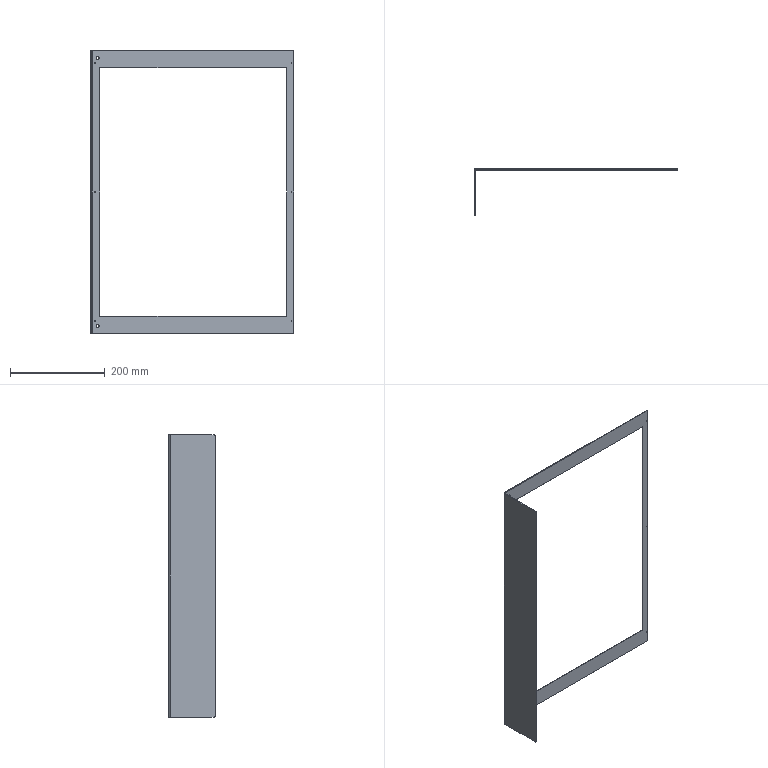Part | NX | features solid 2 | 1 solid | 32 faces | box 430 x 98 x 596 mm | volume 209789 mm3 | cylinder 20 | plane 12 | commonest cylinder face diameters 1 x12 6 x4 5 x2 4 x1 8 x1
STEP:
#1=CARTESIAN_POINT('',(-870.,-1585.,662.5));
#2=VERTEX_POINT('',#1);
#3=CARTESIAN_POINT('',(-870.,-1587.,662.5));
#4=VERTEX_POINT('',#3);
#5=CARTESIAN_POINT('',(-870.,-845.569,662.5));
#6=DIRECTION('',(0.,-1.,0.));
#7=VECTOR('',#6,1000.);
#8=LINE('',#5,#7);
#9=EDGE_CURVE('',#2,#4,#8,.T.);
#10=ORIENTED_EDGE('',*,*,#9,.F.);
#11=CARTESIAN_POINT('',(-870.,-1585.,661.5));
#12=VERTEX_POINT('',#11);
#13=CARTESIAN_POINT('',(-870.,-1585.,662.));
#14=DIRECTION('',(0.,-1.,0.));
#15=DIRECTION('',(0.,0.,-1.));
#16=AXIS2_PLACEMENT_3D('',#13,#14,#15);
#17=CIRCLE('',#16,0.5);
#18=EDGE_CURVE('',#12,#2,#17,.T.);
#19=ORIENTED_EDGE('',*,*,#18,.F.);
#20=CARTESIAN_POINT('',(-870.,-1587.,661.5));
#21=VERTEX_POINT('',#20);
#22=CARTESIAN_POINT('',(-870.,-845.569,661.5));
#23=DIRECTION('',(0.,-1.,0.));
#24=VECTOR('',#23,1000.);
#25=LINE('',#22,#24);
#26=EDGE_CURVE('',#21,#12,#25,.F.);
#27=ORIENTED_EDGE('',*,*,#26,.F.);
#28=CARTESIAN_POINT('',(-870.,-1587.,662.));
#29=DIRECTION('',(0.,-1.,0.));
#30=DIRECTION('',(1.,0.,0.));
#31=AXIS2_PLACEMENT_3D('',#28,#29,#30);
#32=CIRCLE('',#31,0.5);
#33=EDGE_CURVE('',#21,#4,#32,.T.);
#34=ORIENTED_EDGE('',*,*,#33,.T.);
#35=EDGE_LOOP('',(#10,#19,#27,#34));
#36=FACE_BOUND('',#35,.T.);
#37=CARTESIAN_POINT('',(-870.,-845.569,662.));
#38=DIRECTION('',(0.,-1.,0.));
#39=DIRECTION('',(0.,0.,-1.));
#40=AXIS2_PLACEMENT_3D('',#37,#38,#39);
#41=CYLINDRICAL_SURFACE('',#40,0.5);
#42=ADVANCED_FACE('',(#36),#41,.F.);
#43=CARTESIAN_POINT('',(-455.,-1585.,662.5));
#44=VERTEX_POINT('',#43);
#45=CARTESIAN_POINT('',(-455.,-1587.,662.5));
#46=VERTEX_POINT('',#45);
#47=CARTESIAN_POINT('',(-455.,-845.569,662.5));
#48=DIRECTION('',(0.,-1.,0.));
#49=VECTOR('',#48,1000.);
#50=LINE('',#47,#49);
#51=EDGE_CURVE('',#44,#46,#50,.T.);
#52=ORIENTED_EDGE('',*,*,#51,.F.);
#53=CARTESIAN_POINT('',(-455.,-1585.,661.5));
#54=VERTEX_POINT('',#53);
#55=CARTESIAN_POINT('',(-455.,-1585.,662.));
#56=DIRECTION('',(0.,-1.,0.));
#57=DIRECTION('',(0.,0.,-1.));
#58=AXIS2_PLACEMENT_3D('',#55,#56,#57);
#59=CIRCLE('',#58,0.5);
#60=EDGE_CURVE('',#54,#44,#59,.T.);
#61=ORIENTED_EDGE('',*,*,#60,.F.);
#62=CARTESIAN_POINT('',(-455.,-1587.,661.5));
#63=VERTEX_POINT('',#62);
#64=CARTESIAN_POINT('',(-455.,-845.569,661.5));
#65=DIRECTION('',(0.,-1.,0.));
#66=VECTOR('',#65,1000.);
#67=LINE('',#64,#66);
#68=EDGE_CURVE('',#63,#54,#67,.F.);
#69=ORIENTED_EDGE('',*,*,#68,.F.);
#70=CARTESIAN_POINT('',(-455.,-1587.,662.));
#71=DIRECTION('',(0.,-1.,0.));
#72=DIRECTION('',(1.,0.,0.));
#73=AXIS2_PLACEMENT_3D('',#70,#71,#72);
#74=CIRCLE('',#73,0.5);
#75=EDGE_CURVE('',#63,#46,#74,.T.);
#76=ORIENTED_EDGE('',*,*,#75,.T.);
#77=EDGE_LOOP('',(#52,#61,#69,#76));
#78=FACE_BOUND('',#77,.T.);
#79=CARTESIAN_POINT('',(-455.,-845.569,662.));
#80=DIRECTION('',(0.,-1.,0.));
#81=DIRECTION('',(0.,0.,-1.));
#82=AXIS2_PLACEMENT_3D('',#79,#80,#81);
#83=CYLINDRICAL_SURFACE('',#82,0.5);
#84=ADVANCED_FACE('',(#78),#83,.F.);
#85=CARTESIAN_POINT('',(-870.,-1587.,935.5));
#86=VERTEX_POINT('',#85);
#87=CARTESIAN_POINT('',(-870.,-1585.,935.5));
#88=VERTEX_POINT('',#87);
#89=CARTESIAN_POINT('',(-870.,-845.569,935.5));
#90=DIRECTION('',(0.,-1.,0.));
#91=VECTOR('',#90,1000.);
#92=LINE('',#89,#91);
#93=EDGE_CURVE('',#86,#88,#92,.F.);
#94=ORIENTED_EDGE('',*,*,#93,.T.);
#95=CARTESIAN_POINT('',(-870.,-1585.,934.5));
#96=VERTEX_POINT('',#95);
#97=CARTESIAN_POINT('',(-870.,-1585.,935.));
#98=DIRECTION('',(0.,-1.,0.));
#99=DIRECTION('',(0.,0.,-1.));
#100=AXIS2_PLACEMENT_3D('',#97,#98,#99);
#101=CIRCLE('',#100,0.5);
#102=EDGE_CURVE('',#96,#88,#101,.T.);
#103=ORIENTED_EDGE('',*,*,#102,.F.);
#104=CARTESIAN_POINT('',(-870.,-1587.,934.5));
#105=VERTEX_POINT('',#104);
#106=CARTESIAN_POINT('',(-870.,-845.569,934.5));
#107=DIRECTION('',(0.,-1.,0.));
#108=VECTOR('',#107,1000.);
#109=LINE('',#106,#108);
#110=EDGE_CURVE('',#96,#105,#109,.T.);
#111=ORIENTED_EDGE('',*,*,#110,.T.);
#112=CARTESIAN_POINT('',(-870.,-1587.,935.));
#113=DIRECTION('',(0.,-1.,0.));
#114=DIRECTION('',(1.,0.,0.));
#115=AXIS2_PLACEMENT_3D('',#112,#113,#114);
#116=CIRCLE('',#115,0.5);
#117=EDGE_CURVE('',#105,#86,#116,.T.);
#118=ORIENTED_EDGE('',*,*,#117,.T.);
#119=EDGE_LOOP('',(#94,#103,#111,#118));
#120=FACE_BOUND('',#119,.T.);
#121=CARTESIAN_POINT('',(-870.,-845.569,935.));
#122=DIRECTION('',(0.,-1.,0.));
#123=DIRECTION('',(0.,0.,-1.));
#124=AXIS2_PLACEMENT_3D('',#121,#122,#123);
#125=CYLINDRICAL_SURFACE('',#124,0.5);
#126=ADVANCED_FACE('',(#120),#125,.F.);
#127=CARTESIAN_POINT('',(-455.,-1585.,935.5));
#128=VERTEX_POINT('',#127);
#129=CARTESIAN_POINT('',(-455.,-1587.,935.5));
#130=VERTEX_POINT('',#129);
#131=CARTESIAN_POINT('',(-455.,-845.569,935.5));
#132=DIRECTION('',(0.,-1.,0.));
#133=VECTOR('',#132,1000.);
#134=LINE('',#131,#133);
#135=EDGE_CURVE('',#128,#130,#134,.T.);
#136=ORIENTED_EDGE('',*,*,#135,.F.);
#137=CARTESIAN_POINT('',(-455.,-1585.,934.5));
#138=VERTEX_POINT('',#137);
#139=CARTESIAN_POINT('',(-455.,-1585.,935.));
#140=DIRECTION('',(0.,-1.,0.));
#141=DIRECTION('',(0.,0.,-1.));
#142=AXIS2_PLACEMENT_3D('',#139,#140,#141);
#143=CIRCLE('',#142,0.5);
#144=EDGE_CURVE('',#138,#128,#143,.T.);
#145=ORIENTED_EDGE('',*,*,#144,.F.);
#146=CARTESIAN_POINT('',(-455.,-1587.,934.5));
#147=VERTEX_POINT('',#146);
#148=CARTESIAN_POINT('',(-455.,-845.569,934.5));
#149=DIRECTION('',(0.,-1.,0.));
#150=VECTOR('',#149,1000.);
#151=LINE('',#148,#150);
#152=EDGE_CURVE('',#147,#138,#151,.F.);
#153=ORIENTED_EDGE('',*,*,#152,.F.);
#154=CARTESIAN_POINT('',(-455.,-1587.,935.));
#155=DIRECTION('',(0.,-1.,0.));
#156=DIRECTION('',(1.,0.,0.));
#157=AXIS2_PLACEMENT_3D('',#154,#155,#156);
#158=CIRCLE('',#157,0.5);
#159=EDGE_CURVE('',#147,#130,#158,.T.);
#160=ORIENTED_EDGE('',*,*,#159,.T.);
#161=EDGE_LOOP('',(#136,#145,#153,#160));
#162=FACE_BOUND('',#161,.T.);
#163=CARTESIAN_POINT('',(-455.,-845.569,935.));
#164=DIRECTION('',(0.,-1.,0.));
#165=DIRECTION('',(0.,0.,-1.));
#166=AXIS2_PLACEMENT_3D('',#163,#164,#165);
#167=CYLINDRICAL_SURFACE('',#166,0.5);
#168=ADVANCED_FACE('',(#162),#167,.F.);
#169=CARTESIAN_POINT('',(-455.,-1585.,389.5));
#170=VERTEX_POINT('',#169);
#171=CARTESIAN_POINT('',(-455.,-1587.,389.5));
#172=VERTEX_POINT('',#171);
#173=CARTESIAN_POINT('',(-455.,-845.569,389.5));
#174=DIRECTION('',(0.,-1.,0.));
#175=VECTOR('',#174,1000.);
#176=LINE('',#173,#175);
#177=EDGE_CURVE('',#170,#172,#176,.T.);
#178=ORIENTED_EDGE('',*,*,#177,.F.);
#179=CARTESIAN_POINT('',(-455.,-1585.,388.5));
#180=VERTEX_POINT('',#179);
#181=CARTESIAN_POINT('',(-455.,-1585.,389.));
#182=DIRECTION('',(0.,-1.,0.));
#183=DIRECTION('',(0.,0.,-1.));
#184=AXIS2_PLACEMENT_3D('',#181,#182,#183);
#185=CIRCLE('',#184,0.5);
#186=EDGE_CURVE('',#180,#170,#185,.T.);
#187=ORIENTED_EDGE('',*,*,#186,.F.);
#188=CARTESIAN_POINT('',(-455.,-1587.,388.5));
#189=VERTEX_POINT('',#188);
#190=CARTESIAN_POINT('',(-455.,-845.569,388.5));
#191=DIRECTION('',(0.,-1.,0.));
#192=VECTOR('',#191,1000.);
#193=LINE('',#190,#192);
#194=EDGE_CURVE('',#189,#180,#193,.F.);
#195=ORIENTED_EDGE('',*,*,#194,.F.);
#196=CARTESIAN_POINT('',(-455.,-1587.,389.));
#197=DIRECTION('',(0.,-1.,0.));
#198=DIRECTION('',(1.,0.,0.));
#199=AXIS2_PLACEMENT_3D('',#196,#197,#198);
#200=CIRCLE('',#199,0.5);
#201=EDGE_CURVE('',#189,#172,#200,.T.);
#202=ORIENTED_EDGE('',*,*,#201,.T.);
#203=EDGE_LOOP('',(#178,#187,#195,#202));
#204=FACE_BOUND('',#203,.T.);
#205=CARTESIAN_POINT('',(-455.,-845.569,389.));
#206=DIRECTION('',(0.,-1.,0.));
#207=DIRECTION('',(0.,0.,-1.));
#208=AXIS2_PLACEMENT_3D('',#205,#206,#207);
#209=CYLINDRICAL_SURFACE('',#208,0.5);
#210=ADVANCED_FACE('',(#204),#209,.F.);
#211=CARTESIAN_POINT('',(-870.,-1585.,389.5));
#212=VERTEX_POINT('',#211);
#213=CARTESIAN_POINT('',(-870.,-1587.,389.5));
#214=VERTEX_POINT('',#213);
#215=CARTESIAN_POINT('',(-870.,-845.569,389.5));
#216=DIRECTION('',(0.,-1.,0.));
#217=VECTOR('',#216,1000.);
#218=LINE('',#215,#217);
#219=EDGE_CURVE('',#212,#214,#218,.T.);
#220=ORIENTED_EDGE('',*,*,#219,.F.);
#221=CARTESIAN_POINT('',(-870.,-1585.,388.5));
#222=VERTEX_POINT('',#221);
#223=CARTESIAN_POINT('',(-870.,-1585.,389.));
#224=DIRECTION('',(0.,-1.,0.));
#225=DIRECTION('',(0.,0.,-1.));
#226=AXIS2_PLACEMENT_3D('',#223,#224,#225);
#227=CIRCLE('',#226,0.5);
#228=EDGE_CURVE('',#222,#212,#227,.T.);
#229=ORIENTED_EDGE('',*,*,#228,.F.);
#230=CARTESIAN_POINT('',(-870.,-1587.,388.5));
#231=VERTEX_POINT('',#230);
#232=CARTESIAN_POINT('',(-870.,-845.569,388.5));
#233=DIRECTION('',(0.,-1.,0.));
#234=VECTOR('',#233,1000.);
#235=LINE('',#232,#234);
#236=EDGE_CURVE('',#231,#222,#235,.F.);
#237=ORIENTED_EDGE('',*,*,#236,.F.);
#238=CARTESIAN_POINT('',(-870.,-1587.,389.));
#239=DIRECTION('',(0.,-1.,0.));
#240=DIRECTION('',(1.,0.,0.));
#241=AXIS2_PLACEMENT_3D('',#238,#239,#240);
#242=CIRCLE('',#241,0.5);
#243=EDGE_CURVE('',#231,#214,#242,.T.);
#244=ORIENTED_EDGE('',*,*,#243,.T.);
#245=EDGE_LOOP('',(#220,#229,#237,#244));
#246=FACE_BOUND('',#245,.T.);
#247=CARTESIAN_POINT('',(-870.,-845.569,389.));
#248=DIRECTION('',(0.,-1.,0.));
#249=DIRECTION('',(0.,0.,-1.));
#250=AXIS2_PLACEMENT_3D('',#247,#248,#249);
#251=CYLINDRICAL_SURFACE('',#250,0.5);
#252=ADVANCED_FACE('',(#246),#251,.F.);
#253=CARTESIAN_POINT('',(-465.,-1587.,399.));
#254=VERTEX_POINT('',#253);
#255=CARTESIAN_POINT('',(-465.,-1587.,925.));
#256=VERTEX_POINT('',#255);
#257=CARTESIAN_POINT('',(-465.,-1587.,960.));
#258=DIRECTION('',(0.,0.,1.));
#259=VECTOR('',#258,1000.);
#260=LINE('',#257,#259);
#261=EDGE_CURVE('',#254,#256,#260,.T.);
#262=ORIENTED_EDGE('',*,*,#261,.T.);
#263=CARTESIAN_POINT('',(-465.,-1585.,925.));
#264=VERTEX_POINT('',#263);
#265=CARTESIAN_POINT('',(-465.,-2326.431,925.));
#266=DIRECTION('',(0.,1.,0.));
#267=VECTOR('',#266,1000.);
#268=LINE('',#265,#267);
#269=EDGE_CURVE('',#256,#264,#268,.T.);
#270=ORIENTED_EDGE('',*,*,#269,.T.);
#271=CARTESIAN_POINT('',(-465.,-1585.,399.));
#272=VERTEX_POINT('',#271);
#273=CARTESIAN_POINT('',(-465.,-1585.,925.));
#274=DIRECTION('',(0.,0.,-1.));
#275=VECTOR('',#274,1000.);
#276=LINE('',#273,#275);
#277=EDGE_CURVE('',#264,#272,#276,.T.);
#278=ORIENTED_EDGE('',*,*,#277,.T.);
#279=CARTESIAN_POINT('',(-465.,-2326.431,399.));
#280=DIRECTION('',(0.,1.,0.));
#281=VECTOR('',#280,1000.);
#282=LINE('',#279,#281);
#283=EDGE_CURVE('',#254,#272,#282,.T.);
#284=ORIENTED_EDGE('',*,*,#283,.F.);
#285=EDGE_LOOP('',(#262,#270,#278,#284));
#286=FACE_BOUND('',#285,.T.);
#287=CARTESIAN_POINT('',(-465.,-2326.431,925.));
#288=DIRECTION('',(1.,0.,0.));
#289=DIRECTION('',(0.,1.,0.));
#290=AXIS2_PLACEMENT_3D('',#287,#288,#289);
#291=PLANE('',#290);
#292=ADVANCED_FACE('',(#286),#291,.F.);
#293=CARTESIAN_POINT('',(-860.,-1587.,925.));
#294=VERTEX_POINT('',#293);
#295=CARTESIAN_POINT('',(-880.,-1587.,925.));
#296=DIRECTION('',(-1.,0.,0.));
#297=VECTOR('',#296,1000.);
#298=LINE('',#295,#297);
#299=EDGE_CURVE('',#256,#294,#298,.T.);
#300=ORIENTED_EDGE('',*,*,#299,.T.);
#301=CARTESIAN_POINT('',(-860.,-1585.,925.));
#302=VERTEX_POINT('',#301);
#303=CARTESIAN_POINT('',(-860.,-2326.431,925.));
#304=DIRECTION('',(0.,1.,0.));
#305=VECTOR('',#304,1000.);
#306=LINE('',#303,#305);
#307=EDGE_CURVE('',#294,#302,#306,.T.);
#308=ORIENTED_EDGE('',*,*,#307,.T.);
#309=CARTESIAN_POINT('',(-860.,-1585.,925.));
#310=DIRECTION('',(1.,0.,0.));
#311=VECTOR('',#310,1000.);
#312=LINE('',#309,#311);
#313=EDGE_CURVE('',#302,#264,#312,.T.);
#314=ORIENTED_EDGE('',*,*,#313,.T.);
#315=ORIENTED_EDGE('',*,*,#269,.F.);
#316=EDGE_LOOP('',(#300,#308,#314,#315));
#317=FACE_BOUND('',#316,.T.);
#318=CARTESIAN_POINT('',(-860.,-2326.431,925.));
#319=DIRECTION('',(0.,0.,1.));
#320=DIRECTION('',(0.,-1.,0.));
#321=AXIS2_PLACEMENT_3D('',#318,#319,#320);
#322=PLANE('',#321);
#323=ADVANCED_FACE('',(#317),#322,.F.);
#324=CARTESIAN_POINT('',(-860.,-1587.,399.));
#325=VERTEX_POINT('',#324);
#326=CARTESIAN_POINT('',(-860.,-1587.,960.));
#327=DIRECTION('',(0.,0.,-1.));
#328=VECTOR('',#327,1000.);
#329=LINE('',#326,#328);
#330=EDGE_CURVE('',#294,#325,#329,.T.);
#331=ORIENTED_EDGE('',*,*,#330,.T.);
#332=CARTESIAN_POINT('',(-860.,-1585.,399.));
#333=VERTEX_POINT('',#332);
#334=CARTESIAN_POINT('',(-860.,-2326.431,399.));
#335=DIRECTION('',(0.,1.,0.));
#336=VECTOR('',#335,1000.);
#337=LINE('',#334,#336);
#338=EDGE_CURVE('',#325,#333,#337,.T.);
#339=ORIENTED_EDGE('',*,*,#338,.T.);
#340=CARTESIAN_POINT('',(-860.,-1585.,399.));
#341=DIRECTION('',(0.,0.,1.));
#342=VECTOR('',#341,1000.);
#343=LINE('',#340,#342);
#344=EDGE_CURVE('',#333,#302,#343,.T.);
#345=ORIENTED_EDGE('',*,*,#344,.T.);
#346=ORIENTED_EDGE('',*,*,#307,.F.);
#347=EDGE_LOOP('',(#331,#339,#345,#346));
#348=FACE_BOUND('',#347,.T.);
#349=CARTESIAN_POINT('',(-860.,-2326.431,399.));
#350=DIRECTION('',(-1.,0.,0.));
#351=DIRECTION('',(0.,1.,0.));
#352=AXIS2_PLACEMENT_3D('',#349,#350,#351);
#353=PLANE('',#352);
#354=ADVANCED_FACE('',(#348),#353,.F.);
#355=CARTESIAN_POINT('',(-880.,-1587.,399.));
#356=DIRECTION('',(1.,0.,0.));
#357=VECTOR('',#356,1000.);
#358=LINE('',#355,#357);
#359=EDGE_CURVE('',#325,#254,#358,.T.);
#360=ORIENTED_EDGE('',*,*,#359,.T.);
#361=ORIENTED_EDGE('',*,*,#283,.T.);
#362=CARTESIAN_POINT('',(-465.,-1585.,399.));
#363=DIRECTION('',(-1.,0.,0.));
#364=VECTOR('',#363,1000.);
#365=LINE('',#362,#364);
#366=EDGE_CURVE('',#272,#333,#365,.T.);
#367=ORIENTED_EDGE('',*,*,#366,.T.);
#368=ORIENTED_EDGE('',*,*,#338,.F.);
#369=EDGE_LOOP('',(#360,#361,#367,#368));
#370=FACE_BOUND('',#369,.T.);
#371=CARTESIAN_POINT('',(-465.,-2326.431,399.));
#372=DIRECTION('',(0.,0.,-1.));
#373=DIRECTION('',(0.,-1.,0.));
#374=AXIS2_PLACEMENT_3D('',#371,#372,#373);
#375=PLANE('',#374);
#376=ADVANCED_FACE('',(#370),#375,.F.);
#377=CARTESIAN_POINT('',(-864.,-1587.,942.));
#378=VERTEX_POINT('',#377);
#379=CARTESIAN_POINT('',(-864.,-1585.,942.));
#380=VERTEX_POINT('',#379);
#381=CARTESIAN_POINT('',(-864.,-2326.431,942.));
#382=DIRECTION('',(0.,1.,0.));
#383=VECTOR('',#382,1000.);
#384=LINE('',#381,#383);
#385=EDGE_CURVE('',#378,#380,#384,.T.);
#386=ORIENTED_EDGE('',*,*,#385,.F.);
#387=CARTESIAN_POINT('',(-864.,-1587.,948.));
#388=VERTEX_POINT('',#387);
#389=CARTESIAN_POINT('',(-864.,-1587.,945.));
#390=DIRECTION('',(0.,-1.,0.));
#391=DIRECTION('',(0.,0.,-1.));
#392=AXIS2_PLACEMENT_3D('',#389,#390,#391);
#393=CIRCLE('',#392,3.);
#394=EDGE_CURVE('',#378,#388,#393,.T.);
#395=ORIENTED_EDGE('',*,*,#394,.T.);
#396=CARTESIAN_POINT('',(-864.,-1585.,948.));
#397=VERTEX_POINT('',#396);
#398=CARTESIAN_POINT('',(-864.,-2326.431,948.));
#399=DIRECTION('',(0.,1.,0.));
#400=VECTOR('',#399,1000.);
#401=LINE('',#398,#400);
#402=EDGE_CURVE('',#397,#388,#401,.F.);
#403=ORIENTED_EDGE('',*,*,#402,.F.);
#404=CARTESIAN_POINT('',(-864.,-1585.,945.));
#405=DIRECTION('',(0.,1.,0.));
#406=DIRECTION('',(1.,0.,0.));
#407=AXIS2_PLACEMENT_3D('',#404,#405,#406);
#408=CIRCLE('',#407,3.);
#409=EDGE_CURVE('',#397,#380,#408,.T.);
#410=ORIENTED_EDGE('',*,*,#409,.T.);
#411=EDGE_LOOP('',(#386,#395,#403,#410));
#412=FACE_BOUND('',#411,.T.);
#413=CARTESIAN_POINT('',(-864.,-2326.431,945.));
#414=DIRECTION('',(0.,1.,0.));
#415=DIRECTION('',(0.,0.,1.));
#416=AXIS2_PLACEMENT_3D('',#413,#414,#415);
#417=CYLINDRICAL_SURFACE('',#416,3.);
#418=ADVANCED_FACE('',(#412),#417,.F.);
#419=CARTESIAN_POINT('',(-864.,-1585.,376.));
#420=VERTEX_POINT('',#419);
#421=CARTESIAN_POINT('',(-864.,-1587.,376.));
#422=VERTEX_POINT('',#421);
#423=CARTESIAN_POINT('',(-864.,-2326.431,376.));
#424=DIRECTION('',(0.,1.,0.));
#425=VECTOR('',#424,1000.);
#426=LINE('',#423,#425);
#427=EDGE_CURVE('',#420,#422,#426,.F.);
#428=ORIENTED_EDGE('',*,*,#427,.T.);
#429=CARTESIAN_POINT('',(-864.,-1587.,382.));
#430=VERTEX_POINT('',#429);
#431=CARTESIAN_POINT('',(-864.,-1587.,379.));
#432=DIRECTION('',(0.,-1.,0.));
#433=DIRECTION('',(0.,0.,-1.));
#434=AXIS2_PLACEMENT_3D('',#431,#432,#433);
#435=CIRCLE('',#434,3.);
#436=EDGE_CURVE('',#422,#430,#435,.T.);
#437=ORIENTED_EDGE('',*,*,#436,.T.);
#438=CARTESIAN_POINT('',(-864.,-1585.,382.));
#439=VERTEX_POINT('',#438);
#440=CARTESIAN_POINT('',(-864.,-2326.431,382.));
#441=DIRECTION('',(0.,1.,0.));
#442=VECTOR('',#441,1000.);
#443=LINE('',#440,#442);
#444=EDGE_CURVE('',#430,#439,#443,.T.);
#445=ORIENTED_EDGE('',*,*,#444,.T.);
#446=CARTESIAN_POINT('',(-864.,-1585.,379.));
#447=DIRECTION('',(0.,1.,0.));
#448=DIRECTION('',(1.,0.,0.));
#449=AXIS2_PLACEMENT_3D('',#446,#447,#448);
#450=CIRCLE('',#449,3.);
#451=EDGE_CURVE('',#439,#420,#450,.T.);
#452=ORIENTED_EDGE('',*,*,#451,.T.);
#453=EDGE_LOOP('',(#428,#437,#445,#452));
#454=FACE_BOUND('',#453,.T.);
#455=CARTESIAN_POINT('',(-864.,-2326.431,379.));
#456=DIRECTION('',(0.,1.,0.));
#457=DIRECTION('',(0.,0.,1.));
#458=AXIS2_PLACEMENT_3D('',#455,#456,#457);
#459=CYLINDRICAL_SURFACE('',#458,3.);
#460=ADVANCED_FACE('',(#454),#459,.F.);
#461=CARTESIAN_POINT('',(-880.,-1683.,957.5));
#462=VERTEX_POINT('',#461);
#463=CARTESIAN_POINT('',(-880.,-1680.5,960.));
#464=VERTEX_POINT('',#463);
#465=CARTESIAN_POINT('',(-880.,-1680.5,957.5));
#466=DIRECTION('',(-1.,0.,0.));
#467=DIRECTION('',(0.,0.,-1.));
#468=AXIS2_PLACEMENT_3D('',#465,#466,#467);
#469=CIRCLE('',#468,2.5);
#470=EDGE_CURVE('',#462,#464,#469,.T.);
#471=ORIENTED_EDGE('',*,*,#470,.F.);
#472=CARTESIAN_POINT('',(-878.,-1683.,957.5));
#473=VERTEX_POINT('',#472);
#474=CARTESIAN_POINT('',(-880.,-1683.,957.5));
#475=DIRECTION('',(-1.,0.,0.));
#476=VECTOR('',#475,1000.);
#477=LINE('',#474,#476);
#478=EDGE_CURVE('',#473,#462,#477,.T.);
#479=ORIENTED_EDGE('',*,*,#478,.F.);
#480=CARTESIAN_POINT('',(-878.,-1680.5,960.));
#481=VERTEX_POINT('',#480);
#482=CARTESIAN_POINT('',(-878.,-1680.5,957.5));
#483=DIRECTION('',(1.,0.,0.));
#484=DIRECTION('',(0.,0.,-1.));
#485=AXIS2_PLACEMENT_3D('',#482,#483,#484);
#486=CIRCLE('',#485,2.5);
#487=EDGE_CURVE('',#481,#473,#486,.T.);
#488=ORIENTED_EDGE('',*,*,#487,.F.);
#489=CARTESIAN_POINT('',(-880.,-1680.5,960.));
#490=DIRECTION('',(1.,0.,0.));
#491=VECTOR('',#490,1000.);
#492=LINE('',#489,#491);
#493=EDGE_CURVE('',#464,#481,#492,.T.);
#494=ORIENTED_EDGE('',*,*,#493,.F.);
#495=EDGE_LOOP('',(#471,#479,#488,#494));
#496=FACE_BOUND('',#495,.T.);
#497=CARTESIAN_POINT('',(-880.,-1680.5,957.5));
#498=DIRECTION('',(1.,0.,0.));
#499=DIRECTION('',(0.,0.,-1.));
#500=AXIS2_PLACEMENT_3D('',#497,#498,#499);
#501=CYLINDRICAL_SURFACE('',#500,2.5);
#502=ADVANCED_FACE('',(#496),#501,.T.);
#503=CARTESIAN_POINT('',(-880.,-1680.5,364.));
#504=VERTEX_POINT('',#503);
#505=CARTESIAN_POINT('',(-880.,-1683.,366.5));
#506=VERTEX_POINT('',#505);
#507=CARTESIAN_POINT('',(-880.,-1680.5,366.5));
#508=DIRECTION('',(-1.,0.,0.));
#509=DIRECTION('',(0.,0.,-1.));
#510=AXIS2_PLACEMENT_3D('',#507,#508,#509);
#511=CIRCLE('',#510,2.5);
#512=EDGE_CURVE('',#504,#506,#511,.T.);
#513=ORIENTED_EDGE('',*,*,#512,.F.);
#514=CARTESIAN_POINT('',(-878.,-1680.5,364.));
#515=VERTEX_POINT('',#514);
#516=CARTESIAN_POINT('',(-880.,-1680.5,364.));
#517=DIRECTION('',(-1.,0.,0.));
#518=VECTOR('',#517,1000.);
#519=LINE('',#516,#518);
#520=EDGE_CURVE('',#515,#504,#519,.T.);
#521=ORIENTED_EDGE('',*,*,#520,.F.);
#522=CARTESIAN_POINT('',(-878.,-1683.,366.5));
#523=VERTEX_POINT('',#522);
#524=CARTESIAN_POINT('',(-878.,-1680.5,366.5));
#525=DIRECTION('',(1.,0.,0.));
#526=DIRECTION('',(0.,0.,-1.));
#527=AXIS2_PLACEMENT_3D('',#524,#525,#526);
#528=CIRCLE('',#527,2.5);
#529=EDGE_CURVE('',#523,#515,#528,.T.);
#530=ORIENTED_EDGE('',*,*,#529,.F.);
#531=CARTESIAN_POINT('',(-880.,-1683.,366.5));
#532=DIRECTION('',(1.,0.,0.));
#533=VECTOR('',#532,1000.);
#534=LINE('',#531,#533);
#535=EDGE_CURVE('',#506,#523,#534,.T.);
#536=ORIENTED_EDGE('',*,*,#535,.F.);
#537=EDGE_LOOP('',(#513,#521,#530,#536));
#538=FACE_BOUND('',#537,.T.);
#539=CARTESIAN_POINT('',(-880.,-1680.5,366.5));
#540=DIRECTION('',(-1.,0.,0.));
#541=DIRECTION('',(0.,0.,1.));
#542=AXIS2_PLACEMENT_3D('',#539,#540,#541);
#543=CYLINDRICAL_SURFACE('',#542,2.5);
#544=ADVANCED_FACE('',(#538),#543,.T.);
#545=CARTESIAN_POINT('',(-880.,-1683.,960.));
#546=DIRECTION('',(0.,0.,-1.));
#547=VECTOR('',#546,1000.);
#548=LINE('',#545,#547);
#549=EDGE_CURVE('',#462,#506,#548,.T.);
#550=ORIENTED_EDGE('',*,*,#549,.F.);
#551=ORIENTED_EDGE('',*,*,#470,.T.);
#552=CARTESIAN_POINT('',(-880.,-1589.,960.));
#553=VERTEX_POINT('',#552);
#554=CARTESIAN_POINT('',(-880.,-1585.,960.));
#555=DIRECTION('',(0.,-1.,0.));
#556=VECTOR('',#555,1000.);
#557=LINE('',#554,#556);
#558=EDGE_CURVE('',#553,#464,#557,.T.);
#559=ORIENTED_EDGE('',*,*,#558,.F.);
#560=CARTESIAN_POINT('',(-880.,-1589.,364.));
#561=VERTEX_POINT('',#560);
#562=CARTESIAN_POINT('',(-880.,-1589.,960.));
#563=DIRECTION('',(0.,0.,-1.));
#564=VECTOR('',#563,1000.);
#565=LINE('',#562,#564);
#566=EDGE_CURVE('',#553,#561,#565,.T.);
#567=ORIENTED_EDGE('',*,*,#566,.T.);
#568=CARTESIAN_POINT('',(-880.,-1585.,364.));
#569=DIRECTION('',(0.,-1.,0.));
#570=VECTOR('',#569,1000.);
#571=LINE('',#568,#570);
#572=EDGE_CURVE('',#561,#504,#571,.T.);
#573=ORIENTED_EDGE('',*,*,#572,.T.);
#574=ORIENTED_EDGE('',*,*,#512,.T.);
#575=EDGE_LOOP('',(#550,#551,#559,#567,#573,#574));
#576=FACE_BOUND('',#575,.T.);
#577=CARTESIAN_POINT('',(-880.,-1585.,960.));
#578=DIRECTION('',(1.,0.,0.));
#579=DIRECTION('',(0.,1.,0.));
#580=AXIS2_PLACEMENT_3D('',#577,#578,#579);
#581=PLANE('',#580);
#582=ADVANCED_FACE('',(#576),#581,.F.);
#583=CARTESIAN_POINT('',(-876.,-1585.,364.));
#584=VERTEX_POINT('',#583);
#585=CARTESIAN_POINT('',(-876.,-1589.,364.));
#586=DIRECTION('',(0.,0.,1.));
#587=DIRECTION('',(0.,1.,0.));
#588=AXIS2_PLACEMENT_3D('',#585,#586,#587);
#589=CIRCLE('',#588,4.);
#590=EDGE_CURVE('',#584,#561,#589,.T.);
#591=ORIENTED_EDGE('',*,*,#590,.T.);
#592=ORIENTED_EDGE('',*,*,#566,.F.);
#593=CARTESIAN_POINT('',(-876.,-1585.,960.));
#594=VERTEX_POINT('',#593);
#595=CARTESIAN_POINT('',(-876.,-1589.,960.));
#596=DIRECTION('',(0.,0.,1.));
#597=DIRECTION('',(0.,1.,0.));
#598=AXIS2_PLACEMENT_3D('',#595,#596,#597);
#599=CIRCLE('',#598,4.);
#600=EDGE_CURVE('',#594,#553,#599,.T.);
#601=ORIENTED_EDGE('',*,*,#600,.F.);
#602=CARTESIAN_POINT('',(-876.,-1585.,960.));
#603=DIRECTION('',(0.,0.,-1.));
#604=VECTOR('',#603,1000.);
#605=LINE('',#602,#604);
#606=EDGE_CURVE('',#594,#584,#605,.T.);
#607=ORIENTED_EDGE('',*,*,#606,.T.);
#608=EDGE_LOOP('',(#591,#592,#601,#607));
#609=FACE_BOUND('',#608,.T.);
#610=CARTESIAN_POINT('',(-876.,-1589.,960.));
#611=DIRECTION('',(0.,0.,-1.));
#612=DIRECTION('',(0.,1.,0.));
#613=AXIS2_PLACEMENT_3D('',#610,#611,#612);
#614=CYLINDRICAL_SURFACE('',#613,4.);
#615=ADVANCED_FACE('',(#609),#614,.T.);
#616=ORIENTED_EDGE('',*,*,#451,.F.);
#617=CARTESIAN_POINT('',(-864.,-1585.,379.));
#618=DIRECTION('',(0.,1.,0.));
#619=DIRECTION('',(1.,0.,0.));
#620=AXIS2_PLACEMENT_3D('',#617,#618,#619);
#621=CIRCLE('',#620,3.);
#622=EDGE_CURVE('',#420,#439,#621,.T.);
#623=ORIENTED_EDGE('',*,*,#622,.F.);
#624=EDGE_LOOP('',(#616,#623));
#625=FACE_BOUND('',#624,.T.);
#626=ORIENTED_EDGE('',*,*,#409,.F.);
#627=CARTESIAN_POINT('',(-864.,-1585.,945.));
#628=DIRECTION('',(0.,1.,0.));
#629=DIRECTION('',(1.,0.,0.));
#630=AXIS2_PLACEMENT_3D('',#627,#628,#629);
#631=CIRCLE('',#630,3.);
#632=EDGE_CURVE('',#380,#397,#631,.T.);
#633=ORIENTED_EDGE('',*,*,#632,.F.);
#634=EDGE_LOOP('',(#626,#633));
#635=FACE_BOUND('',#634,.T.);
#636=ORIENTED_EDGE('',*,*,#344,.F.);
#637=ORIENTED_EDGE('',*,*,#366,.F.);
#638=ORIENTED_EDGE('',*,*,#277,.F.);
#639=ORIENTED_EDGE('',*,*,#313,.F.);
#640=EDGE_LOOP('',(#636,#637,#638,#639));
#641=FACE_BOUND('',#640,.T.);
#642=ORIENTED_EDGE('',*,*,#228,.T.);
#643=CARTESIAN_POINT('',(-870.,-1585.,389.));
#644=DIRECTION('',(0.,-1.,0.));
#645=DIRECTION('',(0.,0.,-1.));
#646=AXIS2_PLACEMENT_3D('',#643,#644,#645);
#647=CIRCLE('',#646,0.5);
#648=EDGE_CURVE('',#212,#222,#647,.T.);
#649=ORIENTED_EDGE('',*,*,#648,.T.);
#650=EDGE_LOOP('',(#642,#649));
#651=FACE_BOUND('',#650,.T.);
#652=ORIENTED_EDGE('',*,*,#186,.T.);
#653=CARTESIAN_POINT('',(-455.,-1585.,389.));
#654=DIRECTION('',(0.,-1.,0.));
#655=DIRECTION('',(0.,0.,-1.));
#656=AXIS2_PLACEMENT_3D('',#653,#654,#655);
#657=CIRCLE('',#656,0.5);
#658=EDGE_CURVE('',#170,#180,#657,.T.);
#659=ORIENTED_EDGE('',*,*,#658,.T.);
#660=EDGE_LOOP('',(#652,#659));
#661=FACE_BOUND('',#660,.T.);
#662=ORIENTED_EDGE('',*,*,#144,.T.);
#663=CARTESIAN_POINT('',(-455.,-1585.,935.));
#664=DIRECTION('',(0.,-1.,0.));
#665=DIRECTION('',(0.,0.,-1.));
#666=AXIS2_PLACEMENT_3D('',#663,#664,#665);
#667=CIRCLE('',#666,0.5);
#668=EDGE_CURVE('',#128,#138,#667,.T.);
#669=ORIENTED_EDGE('',*,*,#668,.T.);
#670=EDGE_LOOP('',(#662,#669));
#671=FACE_BOUND('',#670,.T.);
#672=ORIENTED_EDGE('',*,*,#102,.T.);
#673=CARTESIAN_POINT('',(-870.,-1585.,935.));
#674=DIRECTION('',(0.,-1.,0.));
#675=DIRECTION('',(0.,0.,-1.));
#676=AXIS2_PLACEMENT_3D('',#673,#674,#675);
#677=CIRCLE('',#676,0.5);
#678=EDGE_CURVE('',#88,#96,#677,.T.);
#679=ORIENTED_EDGE('',*,*,#678,.T.);
#680=EDGE_LOOP('',(#672,#679));
#681=FACE_BOUND('',#680,.T.);
#682=ORIENTED_EDGE('',*,*,#60,.T.);
#683=CARTESIAN_POINT('',(-455.,-1585.,662.));
#684=DIRECTION('',(0.,-1.,0.));
#685=DIRECTION('',(0.,0.,-1.));
#686=AXIS2_PLACEMENT_3D('',#683,#684,#685);
#687=CIRCLE('',#686,0.5);
#688=EDGE_CURVE('',#44,#54,#687,.T.);
#689=ORIENTED_EDGE('',*,*,#688,.T.);
#690=EDGE_LOOP('',(#682,#689));
#691=FACE_BOUND('',#690,.T.);
#692=ORIENTED_EDGE('',*,*,#18,.T.);
#693=CARTESIAN_POINT('',(-870.,-1585.,662.));
#694=DIRECTION('',(0.,-1.,0.));
#695=DIRECTION('',(0.,0.,-1.));
#696=AXIS2_PLACEMENT_3D('',#693,#694,#695);
#697=CIRCLE('',#696,0.5);
#698=EDGE_CURVE('',#2,#12,#697,.T.);
#699=ORIENTED_EDGE('',*,*,#698,.T.);
#700=EDGE_LOOP('',(#692,#699));
#701=FACE_BOUND('',#700,.T.);
#702=CARTESIAN_POINT('',(-450.,-1585.,364.));
#703=VERTEX_POINT('',#702);
#704=CARTESIAN_POINT('',(-880.,-1585.,364.));
#705=DIRECTION('',(-1.,0.,0.));
#706=VECTOR('',#705,1000.);
#707=LINE('',#704,#706);
#708=EDGE_CURVE('',#703,#584,#707,.T.);
#709=ORIENTED_EDGE('',*,*,#708,.T.);
#710=ORIENTED_EDGE('',*,*,#606,.F.);
#711=CARTESIAN_POINT('',(-450.,-1585.,960.));
#712=VERTEX_POINT('',#711);
#713=CARTESIAN_POINT('',(-880.,-1585.,960.));
#714=DIRECTION('',(-1.,0.,0.));
#715=VECTOR('',#714,1000.);
#716=LINE('',#713,#715);
#717=EDGE_CURVE('',#712,#594,#716,.T.);
#718=ORIENTED_EDGE('',*,*,#717,.F.);
#719=CARTESIAN_POINT('',(-450.,-1585.,960.));
#720=DIRECTION('',(0.,0.,-1.));
#721=VECTOR('',#720,1000.);
#722=LINE('',#719,#721);
#723=EDGE_CURVE('',#712,#703,#722,.T.);
#724=ORIENTED_EDGE('',*,*,#723,.T.);
#725=EDGE_LOOP('',(#709,#710,#718,#724));
#726=FACE_BOUND('',#725,.T.);
#727=CARTESIAN_POINT('',(-880.,-1585.,960.));
#728=DIRECTION('',(0.,-1.,0.));
#729=DIRECTION('',(-1.,0.,0.));
#730=AXIS2_PLACEMENT_3D('',#727,#728,#729);
#731=PLANE('',#730);
#732=ADVANCED_FACE('',(#625,#635,#641,#651,#661,#671,#681,#691,#701,#726),#731,.F.);
#733=CARTESIAN_POINT('',(-878.,-1589.,960.));
#734=VERTEX_POINT('',#733);
#735=CARTESIAN_POINT('',(-878.,-1585.,960.));
#736=DIRECTION('',(0.,-1.,0.));
#737=VECTOR('',#736,1000.);
#738=LINE('',#735,#737);
#739=EDGE_CURVE('',#734,#481,#738,.T.);
#740=ORIENTED_EDGE('',*,*,#739,.T.);
#741=ORIENTED_EDGE('',*,*,#487,.T.);
#742=CARTESIAN_POINT('',(-878.,-1683.,960.));
#743=DIRECTION('',(0.,0.,-1.));
#744=VECTOR('',#743,1000.);
#745=LINE('',#742,#744);
#746=EDGE_CURVE('',#473,#523,#745,.T.);
#747=ORIENTED_EDGE('',*,*,#746,.T.);
#748=ORIENTED_EDGE('',*,*,#529,.T.);
#749=CARTESIAN_POINT('',(-878.,-1589.,364.));
#750=VERTEX_POINT('',#749);
#751=CARTESIAN_POINT('',(-878.,-1585.,364.));
#752=DIRECTION('',(0.,-1.,0.));
#753=VECTOR('',#752,1000.);
#754=LINE('',#751,#753);
#755=EDGE_CURVE('',#750,#515,#754,.T.);
#756=ORIENTED_EDGE('',*,*,#755,.F.);
#757=CARTESIAN_POINT('',(-878.,-1589.,960.));
#758=DIRECTION('',(0.,0.,-1.));
#759=VECTOR('',#758,1000.);
#760=LINE('',#757,#759);
#761=EDGE_CURVE('',#734,#750,#760,.T.);
#762=ORIENTED_EDGE('',*,*,#761,.F.);
#763=EDGE_LOOP('',(#740,#741,#747,#748,#756,#762));
#764=FACE_BOUND('',#763,.T.);
#765=CARTESIAN_POINT('',(-878.,-1585.,960.));
#766=DIRECTION('',(1.,0.,0.));
#767=DIRECTION('',(0.,1.,0.));
#768=AXIS2_PLACEMENT_3D('',#765,#766,#767);
#769=PLANE('',#768);
#770=ADVANCED_FACE('',(#764),#769,.T.);
#771=CARTESIAN_POINT('',(-876.,-1587.,364.));
#772=VERTEX_POINT('',#771);
#773=CARTESIAN_POINT('',(-876.,-1589.,364.));
#774=DIRECTION('',(0.,0.,1.));
#775=DIRECTION('',(0.,1.,0.));
#776=AXIS2_PLACEMENT_3D('',#773,#774,#775);
#777=CIRCLE('',#776,2.);
#778=EDGE_CURVE('',#772,#750,#777,.T.);
#779=ORIENTED_EDGE('',*,*,#778,.F.);
#780=CARTESIAN_POINT('',(-876.,-1587.,960.));
#781=VERTEX_POINT('',#780);
#782=CARTESIAN_POINT('',(-876.,-1587.,960.));
#783=DIRECTION('',(0.,0.,-1.));
#784=VECTOR('',#783,1000.);
#785=LINE('',#782,#784);
#786=EDGE_CURVE('',#781,#772,#785,.T.);
#787=ORIENTED_EDGE('',*,*,#786,.F.);
#788=CARTESIAN_POINT('',(-876.,-1589.,960.));
#789=DIRECTION('',(0.,0.,1.));
#790=DIRECTION('',(0.,1.,0.));
#791=AXIS2_PLACEMENT_3D('',#788,#789,#790);
#792=CIRCLE('',#791,2.);
#793=EDGE_CURVE('',#781,#734,#792,.T.);
#794=ORIENTED_EDGE('',*,*,#793,.T.);
#795=ORIENTED_EDGE('',*,*,#761,.T.);
#796=EDGE_LOOP('',(#779,#787,#794,#795));
#797=FACE_BOUND('',#796,.T.);
#798=CARTESIAN_POINT('',(-876.,-1589.,960.));
#799=DIRECTION('',(0.,0.,-1.));
#800=DIRECTION('',(0.,1.,0.));
#801=AXIS2_PLACEMENT_3D('',#798,#799,#800);
#802=CYLINDRICAL_SURFACE('',#801,2.);
#803=ADVANCED_FACE('',(#797),#802,.F.);
#804=CARTESIAN_POINT('',(-864.,-1587.,379.));
#805=DIRECTION('',(0.,-1.,0.));
#806=DIRECTION('',(0.,0.,-1.));
#807=AXIS2_PLACEMENT_3D('',#804,#805,#806);
#808=CIRCLE('',#807,3.);
#809=EDGE_CURVE('',#430,#422,#808,.T.);
#810=ORIENTED_EDGE('',*,*,#809,.F.);
#811=ORIENTED_EDGE('',*,*,#436,.F.);
#812=EDGE_LOOP('',(#810,#811));
#813=FACE_BOUND('',#812,.T.);
#814=CARTESIAN_POINT('',(-864.,-1587.,945.));
#815=DIRECTION('',(0.,-1.,0.));
#816=DIRECTION('',(0.,0.,-1.));
#817=AXIS2_PLACEMENT_3D('',#814,#815,#816);
#818=CIRCLE('',#817,3.);
#819=EDGE_CURVE('',#388,#378,#818,.T.);
#820=ORIENTED_EDGE('',*,*,#819,.F.);
#821=ORIENTED_EDGE('',*,*,#394,.F.);
#822=EDGE_LOOP('',(#820,#821));
#823=FACE_BOUND('',#822,.T.);
#824=ORIENTED_EDGE('',*,*,#359,.F.);
#825=ORIENTED_EDGE('',*,*,#330,.F.);
#826=ORIENTED_EDGE('',*,*,#299,.F.);
#827=ORIENTED_EDGE('',*,*,#261,.F.);
#828=EDGE_LOOP('',(#824,#825,#826,#827));
#829=FACE_BOUND('',#828,.T.);
#830=ORIENTED_EDGE('',*,*,#243,.F.);
#831=CARTESIAN_POINT('',(-870.,-1587.,389.));
#832=DIRECTION('',(0.,-1.,0.));
#833=DIRECTION('',(1.,0.,0.));
#834=AXIS2_PLACEMENT_3D('',#831,#832,#833);
#835=CIRCLE('',#834,0.5);
#836=EDGE_CURVE('',#214,#231,#835,.T.);
#837=ORIENTED_EDGE('',*,*,#836,.F.);
#838=EDGE_LOOP('',(#830,#837));
#839=FACE_BOUND('',#838,.T.);
#840=ORIENTED_EDGE('',*,*,#201,.F.);
#841=CARTESIAN_POINT('',(-455.,-1587.,389.));
#842=DIRECTION('',(0.,-1.,0.));
#843=DIRECTION('',(1.,0.,0.));
#844=AXIS2_PLACEMENT_3D('',#841,#842,#843);
#845=CIRCLE('',#844,0.5);
#846=EDGE_CURVE('',#172,#189,#845,.T.);
#847=ORIENTED_EDGE('',*,*,#846,.F.);
#848=EDGE_LOOP('',(#840,#847));
#849=FACE_BOUND('',#848,.T.);
#850=ORIENTED_EDGE('',*,*,#159,.F.);
#851=CARTESIAN_POINT('',(-455.,-1587.,935.));
#852=DIRECTION('',(0.,-1.,0.));
#853=DIRECTION('',(1.,0.,0.));
#854=AXIS2_PLACEMENT_3D('',#851,#852,#853);
#855=CIRCLE('',#854,0.5);
#856=EDGE_CURVE('',#130,#147,#855,.T.);
#857=ORIENTED_EDGE('',*,*,#856,.F.);
#858=EDGE_LOOP('',(#850,#857));
#859=FACE_BOUND('',#858,.T.);
#860=ORIENTED_EDGE('',*,*,#117,.F.);
#861=CARTESIAN_POINT('',(-870.,-1587.,935.));
#862=DIRECTION('',(0.,-1.,0.));
#863=DIRECTION('',(1.,0.,0.));
#864=AXIS2_PLACEMENT_3D('',#861,#862,#863);
#865=CIRCLE('',#864,0.5);
#866=EDGE_CURVE('',#86,#105,#865,.T.);
#867=ORIENTED_EDGE('',*,*,#866,.F.);
#868=EDGE_LOOP('',(#860,#867));
#869=FACE_BOUND('',#868,.T.);
#870=ORIENTED_EDGE('',*,*,#75,.F.);
#871=CARTESIAN_POINT('',(-455.,-1587.,662.));
#872=DIRECTION('',(0.,-1.,0.));
#873=DIRECTION('',(1.,0.,0.));
#874=AXIS2_PLACEMENT_3D('',#871,#872,#873);
#875=CIRCLE('',#874,0.5);
#876=EDGE_CURVE('',#46,#63,#875,.T.);
#877=ORIENTED_EDGE('',*,*,#876,.F.);
#878=EDGE_LOOP('',(#870,#877));
#879=FACE_BOUND('',#878,.T.);
#880=ORIENTED_EDGE('',*,*,#33,.F.);
#881=CARTESIAN_POINT('',(-870.,-1587.,662.));
#882=DIRECTION('',(0.,-1.,0.));
#883=DIRECTION('',(1.,0.,0.));
#884=AXIS2_PLACEMENT_3D('',#881,#882,#883);
#885=CIRCLE('',#884,0.5);
#886=EDGE_CURVE('',#4,#21,#885,.T.);
#887=ORIENTED_EDGE('',*,*,#886,.F.);
#888=EDGE_LOOP('',(#880,#887));
#889=FACE_BOUND('',#888,.T.);
#890=CARTESIAN_POINT('',(-450.,-1587.,364.));
#891=VERTEX_POINT('',#890);
#892=CARTESIAN_POINT('',(-880.,-1587.,364.));
#893=DIRECTION('',(-1.,0.,0.));
#894=VECTOR('',#893,1000.);
#895=LINE('',#892,#894);
#896=EDGE_CURVE('',#891,#772,#895,.T.);
#897=ORIENTED_EDGE('',*,*,#896,.F.);
#898=CARTESIAN_POINT('',(-450.,-1587.,960.));
#899=VERTEX_POINT('',#898);
#900=CARTESIAN_POINT('',(-450.,-1587.,960.));
#901=DIRECTION('',(0.,0.,-1.));
#902=VECTOR('',#901,1000.);
#903=LINE('',#900,#902);
#904=EDGE_CURVE('',#899,#891,#903,.T.);
#905=ORIENTED_EDGE('',*,*,#904,.F.);
#906=CARTESIAN_POINT('',(-880.,-1587.,960.));
#907=DIRECTION('',(-1.,0.,0.));
#908=VECTOR('',#907,1000.);
#909=LINE('',#906,#908);
#910=EDGE_CURVE('',#899,#781,#909,.T.);
#911=ORIENTED_EDGE('',*,*,#910,.T.);
#912=ORIENTED_EDGE('',*,*,#786,.T.);
#913=EDGE_LOOP('',(#897,#905,#911,#912));
#914=FACE_BOUND('',#913,.T.);
#915=CARTESIAN_POINT('',(-880.,-1587.,960.));
#916=DIRECTION('',(0.,-1.,0.));
#917=DIRECTION('',(-1.,0.,0.));
#918=AXIS2_PLACEMENT_3D('',#915,#916,#917);
#919=PLANE('',#918);
#920=ADVANCED_FACE('',(#813,#823,#829,#839,#849,#859,#869,#879,#889,#914),#919,.T.);
#921=ORIENTED_EDGE('',*,*,#723,.F.);
#922=CARTESIAN_POINT('',(-450.,-1585.,960.));
#923=DIRECTION('',(0.,-1.,0.));
#924=VECTOR('',#923,1000.);
#925=LINE('',#922,#924);
#926=EDGE_CURVE('',#712,#899,#925,.T.);
#927=ORIENTED_EDGE('',*,*,#926,.T.);
#928=ORIENTED_EDGE('',*,*,#904,.T.);
#929=CARTESIAN_POINT('',(-450.,-1585.,364.));
#930=DIRECTION('',(0.,-1.,0.));
#931=VECTOR('',#930,1000.);
#932=LINE('',#929,#931);
#933=EDGE_CURVE('',#703,#891,#932,.T.);
#934=ORIENTED_EDGE('',*,*,#933,.F.);
#935=EDGE_LOOP('',(#921,#927,#928,#934));
#936=FACE_BOUND('',#935,.T.);
#937=CARTESIAN_POINT('',(-450.,-1585.,960.));
#938=DIRECTION('',(-1.,0.,0.));
#939=DIRECTION('',(0.,1.,0.));
#940=AXIS2_PLACEMENT_3D('',#937,#938,#939);
#941=PLANE('',#940);
#942=ADVANCED_FACE('',(#936),#941,.F.);
#943=ORIENTED_EDGE('',*,*,#755,.T.);
#944=ORIENTED_EDGE('',*,*,#520,.T.);
#945=ORIENTED_EDGE('',*,*,#572,.F.);
#946=ORIENTED_EDGE('',*,*,#590,.F.);
#947=ORIENTED_EDGE('',*,*,#708,.F.);
#948=ORIENTED_EDGE('',*,*,#933,.T.);
#949=ORIENTED_EDGE('',*,*,#896,.T.);
#950=ORIENTED_EDGE('',*,*,#778,.T.);
#951=EDGE_LOOP('',(#943,#944,#945,#946,#947,#948,#949,#950));
#952=FACE_BOUND('',#951,.T.);
#953=CARTESIAN_POINT('',(-880.,-1585.,364.));
#954=DIRECTION('',(0.,0.,1.));
#955=DIRECTION('',(0.,-1.,0.));
#956=AXIS2_PLACEMENT_3D('',#953,#954,#955);
#957=PLANE('',#956);
#958=ADVANCED_FACE('',(#952),#957,.F.);
#959=ORIENTED_EDGE('',*,*,#746,.F.);
#960=ORIENTED_EDGE('',*,*,#478,.T.);
#961=ORIENTED_EDGE('',*,*,#549,.T.);
#962=ORIENTED_EDGE('',*,*,#535,.T.);
#963=EDGE_LOOP('',(#959,#960,#961,#962));
#964=FACE_BOUND('',#963,.T.);
#965=CARTESIAN_POINT('',(-880.,-1683.,960.));
#966=DIRECTION('',(0.,-1.,0.));
#967=DIRECTION('',(-1.,0.,0.));
#968=AXIS2_PLACEMENT_3D('',#965,#966,#967);
#969=PLANE('',#968);
#970=ADVANCED_FACE('',(#964),#969,.T.);
#971=ORIENTED_EDGE('',*,*,#558,.T.);
#972=ORIENTED_EDGE('',*,*,#493,.T.);
#973=ORIENTED_EDGE('',*,*,#739,.F.);
#974=ORIENTED_EDGE('',*,*,#793,.F.);
#975=ORIENTED_EDGE('',*,*,#910,.F.);
#976=ORIENTED_EDGE('',*,*,#926,.F.);
#977=ORIENTED_EDGE('',*,*,#717,.T.);
#978=ORIENTED_EDGE('',*,*,#600,.T.);
#979=EDGE_LOOP('',(#971,#972,#973,#974,#975,#976,#977,#978));
#980=FACE_BOUND('',#979,.T.);
#981=CARTESIAN_POINT('',(-880.,-1585.,960.));
#982=DIRECTION('',(0.,0.,1.));
#983=DIRECTION('',(0.,-1.,0.));
#984=AXIS2_PLACEMENT_3D('',#981,#982,#983);
#985=PLANE('',#984);
#986=ADVANCED_FACE('',(#980),#985,.T.);
#987=ORIENTED_EDGE('',*,*,#809,.T.);
#988=ORIENTED_EDGE('',*,*,#427,.F.);
#989=ORIENTED_EDGE('',*,*,#622,.T.);
#990=ORIENTED_EDGE('',*,*,#444,.F.);
#991=EDGE_LOOP('',(#987,#988,#989,#990));
#992=FACE_BOUND('',#991,.T.);
#993=CARTESIAN_POINT('',(-864.,-2326.431,379.));
#994=DIRECTION('',(0.,1.,0.));
#995=DIRECTION('',(0.,0.,1.));
#996=AXIS2_PLACEMENT_3D('',#993,#994,#995);
#997=CYLINDRICAL_SURFACE('',#996,3.);
#998=ADVANCED_FACE('',(#992),#997,.F.);
#999=ORIENTED_EDGE('',*,*,#819,.T.);
#1000=ORIENTED_EDGE('',*,*,#385,.T.);
#1001=ORIENTED_EDGE('',*,*,#632,.T.);
#1002=ORIENTED_EDGE('',*,*,#402,.T.);
#1003=EDGE_LOOP('',(#999,#1000,#1001,#1002));
#1004=FACE_BOUND('',#1003,.T.);
#1005=CARTESIAN_POINT('',(-864.,-2326.431,945.));
#1006=DIRECTION('',(0.,1.,0.));
#1007=DIRECTION('',(0.,0.,1.));
#1008=AXIS2_PLACEMENT_3D('',#1005,#1006,#1007);
#1009=CYLINDRICAL_SURFACE('',#1008,3.);
#1010=ADVANCED_FACE('',(#1004),#1009,.F.);
#1011=ORIENTED_EDGE('',*,*,#648,.F.);
#1012=ORIENTED_EDGE('',*,*,#219,.T.);
#1013=ORIENTED_EDGE('',*,*,#836,.T.);
#1014=ORIENTED_EDGE('',*,*,#236,.T.);
#1015=EDGE_LOOP('',(#1011,#1012,#1013,#1014));
#1016=FACE_BOUND('',#1015,.T.);
#1017=CARTESIAN_POINT('',(-870.,-845.569,389.));
#1018=DIRECTION('',(0.,-1.,0.));
#1019=DIRECTION('',(0.,0.,-1.));
#1020=AXIS2_PLACEMENT_3D('',#1017,#1018,#1019);
#1021=CYLINDRICAL_SURFACE('',#1020,0.5);
#1022=ADVANCED_FACE('',(#1016),#1021,.F.);
#1023=ORIENTED_EDGE('',*,*,#658,.F.);
#1024=ORIENTED_EDGE('',*,*,#177,.T.);
#1025=ORIENTED_EDGE('',*,*,#846,.T.);
#1026=ORIENTED_EDGE('',*,*,#194,.T.);
#1027=EDGE_LOOP('',(#1023,#1024,#1025,#1026));
#1028=FACE_BOUND('',#1027,.T.);
#1029=CARTESIAN_POINT('',(-455.,-845.569,389.));
#1030=DIRECTION('',(0.,-1.,0.));
#1031=DIRECTION('',(0.,0.,-1.));
#1032=AXIS2_PLACEMENT_3D('',#1029,#1030,#1031);
#1033=CYLINDRICAL_SURFACE('',#1032,0.5);
#1034=ADVANCED_FACE('',(#1028),#1033,.F.);
#1035=ORIENTED_EDGE('',*,*,#668,.F.);
#1036=ORIENTED_EDGE('',*,*,#135,.T.);
#1037=ORIENTED_EDGE('',*,*,#856,.T.);
#1038=ORIENTED_EDGE('',*,*,#152,.T.);
#1039=EDGE_LOOP('',(#1035,#1036,#1037,#1038));
#1040=FACE_BOUND('',#1039,.T.);
#1041=CARTESIAN_POINT('',(-455.,-845.569,935.));
#1042=DIRECTION('',(0.,-1.,0.));
#1043=DIRECTION('',(0.,0.,-1.));
#1044=AXIS2_PLACEMENT_3D('',#1041,#1042,#1043);
#1045=CYLINDRICAL_SURFACE('',#1044,0.5);
#1046=ADVANCED_FACE('',(#1040),#1045,.F.);
#1047=ORIENTED_EDGE('',*,*,#678,.F.);
#1048=ORIENTED_EDGE('',*,*,#93,.F.);
#1049=ORIENTED_EDGE('',*,*,#866,.T.);
#1050=ORIENTED_EDGE('',*,*,#110,.F.);
#1051=EDGE_LOOP('',(#1047,#1048,#1049,#1050));
#1052=FACE_BOUND('',#1051,.T.);
#1053=CARTESIAN_POINT('',(-870.,-845.569,935.));
#1054=DIRECTION('',(0.,-1.,0.));
#1055=DIRECTION('',(0.,0.,-1.));
#1056=AXIS2_PLACEMENT_3D('',#1053,#1054,#1055);
#1057=CYLINDRICAL_SURFACE('',#1056,0.5);
#1058=ADVANCED_FACE('',(#1052),#1057,.F.);
#1059=ORIENTED_EDGE('',*,*,#688,.F.);
#1060=ORIENTED_EDGE('',*,*,#51,.T.);
#1061=ORIENTED_EDGE('',*,*,#876,.T.);
#1062=ORIENTED_EDGE('',*,*,#68,.T.);
#1063=EDGE_LOOP('',(#1059,#1060,#1061,#1062));
#1064=FACE_BOUND('',#1063,.T.);
#1065=CARTESIAN_POINT('',(-455.,-845.569,662.));
#1066=DIRECTION('',(0.,-1.,0.));
#1067=DIRECTION('',(0.,0.,-1.));
#1068=AXIS2_PLACEMENT_3D('',#1065,#1066,#1067);
#1069=CYLINDRICAL_SURFACE('',#1068,0.5);
#1070=ADVANCED_FACE('',(#1064),#1069,.F.);
#1071=ORIENTED_EDGE('',*,*,#698,.F.);
#1072=ORIENTED_EDGE('',*,*,#9,.T.);
#1073=ORIENTED_EDGE('',*,*,#886,.T.);
#1074=ORIENTED_EDGE('',*,*,#26,.T.);
#1075=EDGE_LOOP('',(#1071,#1072,#1073,#1074));
#1076=FACE_BOUND('',#1075,.T.);
#1077=CARTESIAN_POINT('',(-870.,-845.569,662.));
#1078=DIRECTION('',(0.,-1.,0.));
#1079=DIRECTION('',(0.,0.,-1.));
#1080=AXIS2_PLACEMENT_3D('',#1077,#1078,#1079);
#1081=CYLINDRICAL_SURFACE('',#1080,0.5);
#1082=ADVANCED_FACE('',(#1076),#1081,.F.);
#1083=CLOSED_SHELL('',(#42,#84,#126,#168,#210,#252,#292,#323,#354,#376,#418,#460,#502,#544,#582,#615,#732,#770,#803,#920,#942,#958,#970,#986,#998,#1010,#1022,#1034,#1046,#1058,#1070,#1082));
#1084=MANIFOLD_SOLID_BREP('',#1083);
#1085=(LENGTH_UNIT()NAMED_UNIT(*)SI_UNIT(.MILLI.,.METRE.));
#1086=UNCERTAINTY_MEASURE_WITH_UNIT(LENGTH_MEASURE(0.00001),#1085,'','');
#1087=(NAMED_UNIT(*)PLANE_ANGLE_UNIT()SI_UNIT($,.RADIAN.));
#1088=(NAMED_UNIT(*)SI_UNIT($,.STERADIAN.)SOLID_ANGLE_UNIT());
#1089=(GEOMETRIC_REPRESENTATION_CONTEXT(3)GLOBAL_UNCERTAINTY_ASSIGNED_CONTEXT((#1086))GLOBAL_UNIT_ASSIGNED_CONTEXT((#1085,#1087,#1088))REPRESENTATION_CONTEXT('',''));
#1090=ADVANCED_BREP_SHAPE_REPRESENTATION('',(#1084),#1089);